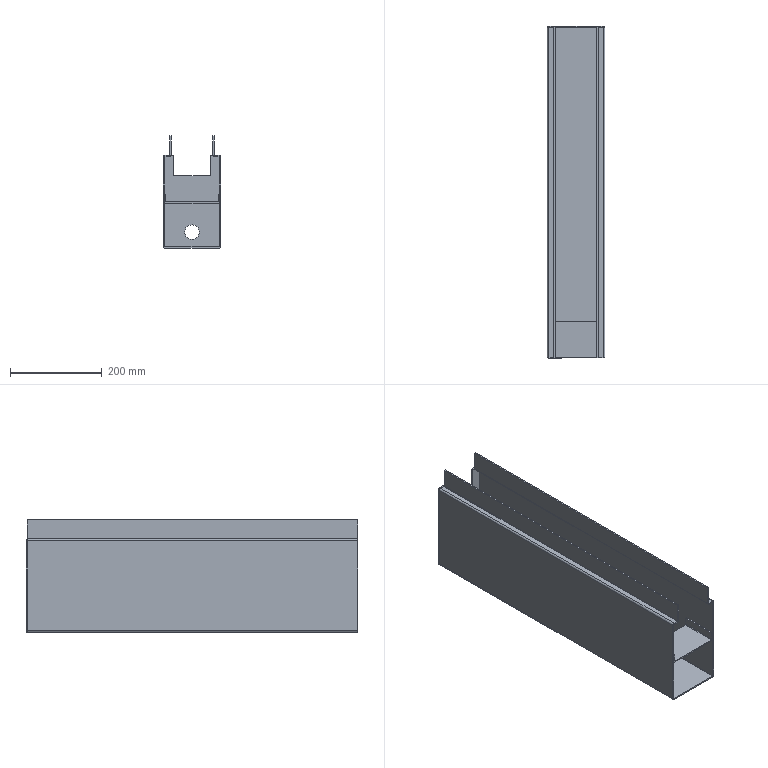Part | STEP file | X77-08303 | 3 solids | 84 faces | box 126 x 723 x 245 mm | volume 1470130 mm3 | plane 62 | cylinder 22 | commonest cylinder face diameters 7.473 x10 1.473 x6 2 x2 6 x2 32 x2